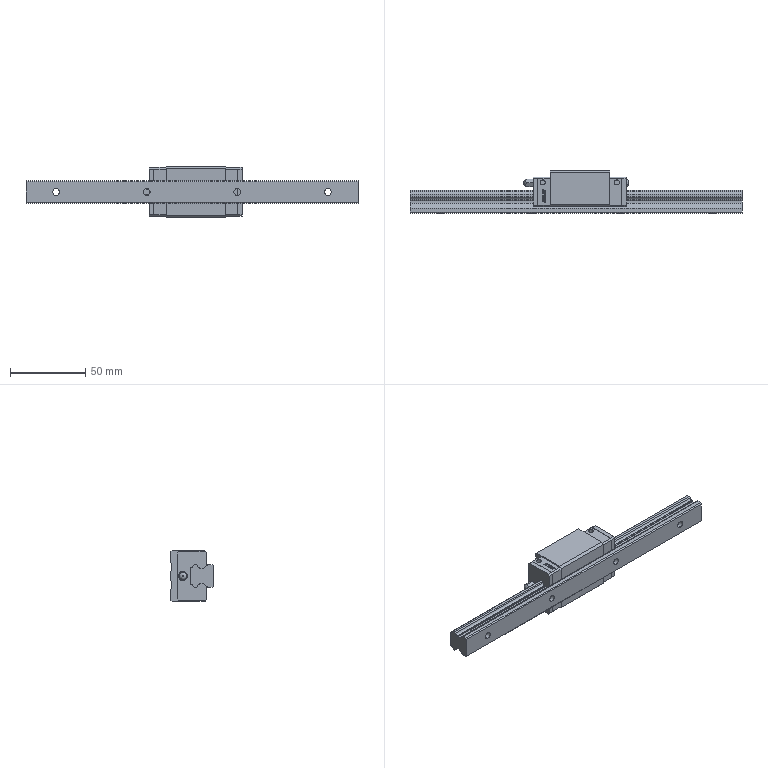Part | SolidWorks | features AEMSimFeature 1 | 8 solids | 813 faces | box 220 x 28 x 34 mm | volume 77398 mm3 | plane 588 | cylinder 132 | spline 59 | cone 32 | sphere 2 | commonest cylinder face diameters 0.8 x48 3.24 x24 4 x12 3.242 x8 3.3 x8 4.5 x8